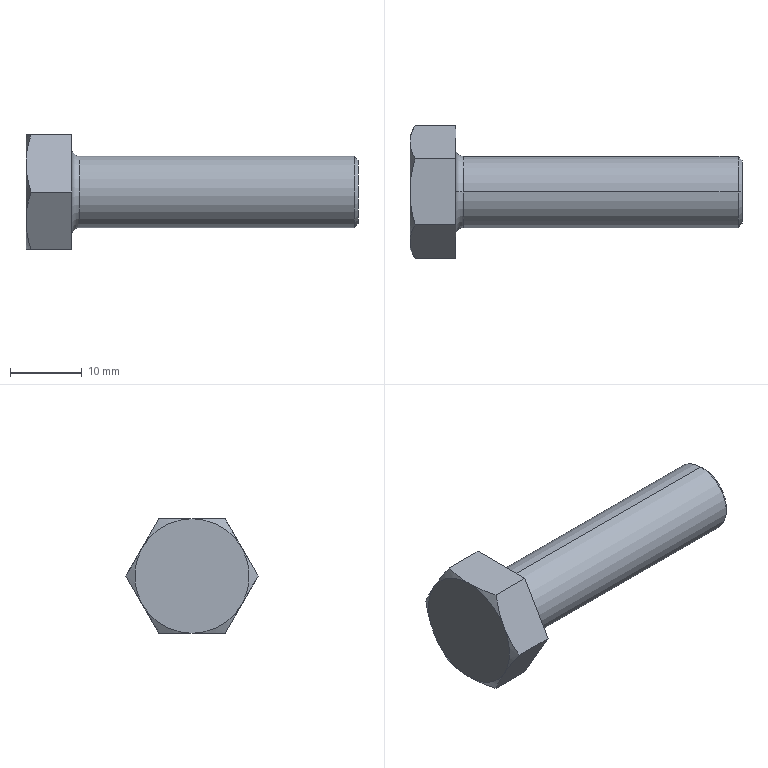Part | SolidWorks | features Chamfer 2, RevCut 2, Revolution 2, Extrusion 1, ICE 1 | 1 solid | 21 faces | box 46.4 x 18.475 x 16 mm | volume 4560 mm3 | plane 9 | cone 8 | cylinder 2 | torus 2 | commonest cylinder face diameters 10 x2
STEP:
#1=CARTESIAN_POINT('',(46.4,0.,-4.444));
#2=VERTEX_POINT('',#1);
#3=CARTESIAN_POINT('',(46.4,0.,4.444));
#4=VERTEX_POINT('',#3);
#5=CARTESIAN_POINT('',(46.4,0.,0.));
#6=DIRECTION('',(1.,0.,0.));
#7=DIRECTION('',(0.,0.,1.));
#8=AXIS2_PLACEMENT_3D('',#5,#6,#7);
#9=CIRCLE('',#8,4.444);
#10=EDGE_CURVE('',#2,#4,#9,.T.);
#11=ORIENTED_EDGE('',*,*,#10,.F.);
#12=CARTESIAN_POINT('',(45.844,0.,-5.));
#13=VERTEX_POINT('',#12);
#14=CARTESIAN_POINT('',(45.844,0.,-5.));
#15=DIRECTION('',(-0.7071,0.,-0.7071));
#16=VECTOR('',#15,1000.);
#17=LINE('',#14,#16);
#18=EDGE_CURVE('',#2,#13,#17,.T.);
#19=ORIENTED_EDGE('',*,*,#18,.T.);
#20=CARTESIAN_POINT('',(45.844,0.,5.));
#21=VERTEX_POINT('',#20);
#22=CARTESIAN_POINT('',(45.844,0.,0.));
#23=DIRECTION('',(-1.,0.,0.));
#24=DIRECTION('',(0.,0.,1.));
#25=AXIS2_PLACEMENT_3D('',#22,#23,#24);
#26=CIRCLE('',#25,5.);
#27=EDGE_CURVE('',#21,#13,#26,.T.);
#28=ORIENTED_EDGE('',*,*,#27,.F.);
#29=CARTESIAN_POINT('',(45.844,0.,5.));
#30=DIRECTION('',(-0.7071,0.,0.7071));
#31=VECTOR('',#30,1000.);
#32=LINE('',#29,#31);
#33=EDGE_CURVE('',#4,#21,#32,.T.);
#34=ORIENTED_EDGE('',*,*,#33,.F.);
#35=EDGE_LOOP('',(#11,#19,#28,#34));
#36=FACE_OUTER_BOUND('',#35,.T.);
#37=CARTESIAN_POINT('',(45.844,0.,0.));
#38=DIRECTION('',(-1.,0.,0.));
#39=DIRECTION('',(0.,0.,1.));
#40=AXIS2_PLACEMENT_3D('',#37,#38,#39);
#41=CONICAL_SURFACE('',#40,5.,0.7854);
#42=ADVANCED_FACE('',(#36),#41,.T.);
#43=ORIENTED_EDGE('',*,*,#27,.T.);
#44=CARTESIAN_POINT('',(7.5,0.,-5.));
#45=VERTEX_POINT('',#44);
#46=CARTESIAN_POINT('',(6.4,0.,-5.));
#47=DIRECTION('',(-1.,0.,0.));
#48=VECTOR('',#47,1000.);
#49=LINE('',#46,#48);
#50=EDGE_CURVE('',#13,#45,#49,.T.);
#51=ORIENTED_EDGE('',*,*,#50,.T.);
#52=CARTESIAN_POINT('',(7.5,0.,5.));
#53=VERTEX_POINT('',#52);
#54=CARTESIAN_POINT('',(7.5,0.,0.));
#55=DIRECTION('',(-1.,0.,0.));
#56=DIRECTION('',(0.,0.,1.));
#57=AXIS2_PLACEMENT_3D('',#54,#55,#56);
#58=CIRCLE('',#57,5.);
#59=EDGE_CURVE('',#53,#45,#58,.T.);
#60=ORIENTED_EDGE('',*,*,#59,.F.);
#61=CARTESIAN_POINT('',(6.4,0.,5.));
#62=DIRECTION('',(-1.,0.,0.));
#63=VECTOR('',#62,1000.);
#64=LINE('',#61,#63);
#65=EDGE_CURVE('',#21,#53,#64,.T.);
#66=ORIENTED_EDGE('',*,*,#65,.F.);
#67=EDGE_LOOP('',(#43,#51,#60,#66));
#68=FACE_OUTER_BOUND('',#67,.T.);
#69=CARTESIAN_POINT('',(6.4,0.,0.));
#70=DIRECTION('',(-1.,0.,0.));
#71=DIRECTION('',(0.,0.,1.));
#72=AXIS2_PLACEMENT_3D('',#69,#70,#71);
#73=CYLINDRICAL_SURFACE('',#72,5.);
#74=ADVANCED_FACE('',(#68),#73,.T.);
#75=CARTESIAN_POINT('',(6.4,0.,-6.1));
#76=VERTEX_POINT('',#75);
#77=CARTESIAN_POINT('',(6.4,0.,6.1));
#78=VERTEX_POINT('',#77);
#79=CARTESIAN_POINT('',(6.4,0.,0.));
#80=DIRECTION('',(-1.,0.,0.));
#81=DIRECTION('',(0.,0.,1.));
#82=AXIS2_PLACEMENT_3D('',#79,#80,#81);
#83=CIRCLE('',#82,6.1);
#84=EDGE_CURVE('',#76,#78,#83,.T.);
#85=ORIENTED_EDGE('',*,*,#84,.F.);
#86=CARTESIAN_POINT('',(7.5,0.,-6.1));
#87=DIRECTION('',(0.,1.,0.));
#88=DIRECTION('',(0.,0.,1.));
#89=AXIS2_PLACEMENT_3D('',#86,#87,#88);
#90=CIRCLE('',#89,1.1);
#91=EDGE_CURVE('',#76,#45,#90,.T.);
#92=ORIENTED_EDGE('',*,*,#91,.T.);
#93=CARTESIAN_POINT('',(7.5,0.,0.));
#94=DIRECTION('',(-1.,0.,0.));
#95=DIRECTION('',(0.,0.,1.));
#96=AXIS2_PLACEMENT_3D('',#93,#94,#95);
#97=CIRCLE('',#96,5.);
#98=EDGE_CURVE('',#45,#53,#97,.T.);
#99=ORIENTED_EDGE('',*,*,#98,.T.);
#100=CARTESIAN_POINT('',(7.5,0.,6.1));
#101=DIRECTION('',(0.,-1.,0.));
#102=DIRECTION('',(0.,0.,-1.));
#103=AXIS2_PLACEMENT_3D('',#100,#101,#102);
#104=CIRCLE('',#103,1.1);
#105=EDGE_CURVE('',#78,#53,#104,.T.);
#106=ORIENTED_EDGE('',*,*,#105,.F.);
#107=EDGE_LOOP('',(#85,#92,#99,#106));
#108=FACE_OUTER_BOUND('',#107,.T.);
#109=CARTESIAN_POINT('',(7.5,0.,0.));
#110=DIRECTION('',(-1.,0.,0.));
#111=DIRECTION('',(0.,0.,1.));
#112=AXIS2_PLACEMENT_3D('',#109,#110,#111);
#113=TOROIDAL_SURFACE('',#112,6.1,1.1);
#114=ADVANCED_FACE('',(#108),#113,.F.);
#115=CARTESIAN_POINT('',(6.4,-4.619,-8.));
#116=VERTEX_POINT('',#115);
#117=CARTESIAN_POINT('',(6.4,4.619,-8.));
#118=VERTEX_POINT('',#117);
#119=CARTESIAN_POINT('',(6.4,-4.619,-8.));
#120=DIRECTION('',(0.,1.,0.));
#121=VECTOR('',#120,1000.);
#122=LINE('',#119,#121);
#123=EDGE_CURVE('',#116,#118,#122,.T.);
#124=ORIENTED_EDGE('',*,*,#123,.T.);
#125=CARTESIAN_POINT('',(6.4,9.238,0.));
#126=VERTEX_POINT('',#125);
#127=CARTESIAN_POINT('',(6.4,4.619,-8.));
#128=DIRECTION('',(0.,0.5,0.866));
#129=VECTOR('',#128,1000.);
#130=LINE('',#127,#129);
#131=EDGE_CURVE('',#118,#126,#130,.T.);
#132=ORIENTED_EDGE('',*,*,#131,.T.);
#133=CARTESIAN_POINT('',(6.4,4.619,8.));
#134=VERTEX_POINT('',#133);
#135=CARTESIAN_POINT('',(6.4,9.238,0.));
#136=DIRECTION('',(0.,-0.5,0.866));
#137=VECTOR('',#136,1000.);
#138=LINE('',#135,#137);
#139=EDGE_CURVE('',#126,#134,#138,.T.);
#140=ORIENTED_EDGE('',*,*,#139,.T.);
#141=CARTESIAN_POINT('',(6.4,-4.619,8.));
#142=VERTEX_POINT('',#141);
#143=CARTESIAN_POINT('',(6.4,4.619,8.));
#144=DIRECTION('',(0.,-1.,0.));
#145=VECTOR('',#144,1000.);
#146=LINE('',#143,#145);
#147=EDGE_CURVE('',#134,#142,#146,.T.);
#148=ORIENTED_EDGE('',*,*,#147,.T.);
#149=CARTESIAN_POINT('',(6.4,-9.238,0.));
#150=VERTEX_POINT('',#149);
#151=CARTESIAN_POINT('',(6.4,-4.619,8.));
#152=DIRECTION('',(0.,-0.5,-0.866));
#153=VECTOR('',#152,1000.);
#154=LINE('',#151,#153);
#155=EDGE_CURVE('',#142,#150,#154,.T.);
#156=ORIENTED_EDGE('',*,*,#155,.T.);
#157=CARTESIAN_POINT('',(6.4,-9.238,0.));
#158=DIRECTION('',(0.,0.5,-0.866));
#159=VECTOR('',#158,1000.);
#160=LINE('',#157,#159);
#161=EDGE_CURVE('',#150,#116,#160,.T.);
#162=ORIENTED_EDGE('',*,*,#161,.T.);
#163=EDGE_LOOP('',(#124,#132,#140,#148,#156,#162));
#164=FACE_OUTER_BOUND('',#163,.T.);
#165=CARTESIAN_POINT('',(6.4,0.,0.));
#166=DIRECTION('',(-1.,0.,0.));
#167=DIRECTION('',(0.,0.,1.));
#168=AXIS2_PLACEMENT_3D('',#165,#166,#167);
#169=CIRCLE('',#168,6.1);
#170=EDGE_CURVE('',#78,#76,#169,.T.);
#171=ORIENTED_EDGE('',*,*,#170,.T.);
#172=ORIENTED_EDGE('',*,*,#84,.T.);
#173=EDGE_LOOP('',(#171,#172));
#174=FACE_BOUND('',#173,.T.);
#175=CARTESIAN_POINT('',(6.4,4.619,-8.));
#176=DIRECTION('',(1.,0.,0.));
#177=DIRECTION('',(0.,0.,-1.));
#178=AXIS2_PLACEMENT_3D('',#175,#176,#177);
#179=PLANE('',#178);
#180=ADVANCED_FACE('',(#164,#174),#179,.T.);
#181=CARTESIAN_POINT('',(0.7145,4.619,-8.));
#182=VERTEX_POINT('',#181);
#183=CARTESIAN_POINT('',(0.,0.,-8.));
#184=VERTEX_POINT('',#183);
#185=CARTESIAN_POINT('',(0.7145,4.619,-8.));
#186=CARTESIAN_POINT('',(0.4989,3.872,-8.));
#187=CARTESIAN_POINT('',(0.3194,3.115,-8.));
#188=CARTESIAN_POINT('',(0.06895,1.573,-8.));
#189=CARTESIAN_POINT('',(0.,0.781,-8.));
#190=CARTESIAN_POINT('',(0.,0.,-8.));
#191=B_SPLINE_CURVE_WITH_KNOTS('',3,(#185,#186,#187,#188,#189,#190),.UNSPECIFIED.,.F.,.F.,(4,2,4),(0.003372,0.005703,0.008035),.UNSPECIFIED.);
#192=EDGE_CURVE('',#182,#184,#191,.T.);
#193=ORIENTED_EDGE('',*,*,#192,.F.);
#194=CARTESIAN_POINT('',(6.4,4.619,-8.));
#195=DIRECTION('',(-1.,0.,0.));
#196=VECTOR('',#195,1000.);
#197=LINE('',#194,#196);
#198=EDGE_CURVE('',#118,#182,#197,.T.);
#199=ORIENTED_EDGE('',*,*,#198,.F.);
#200=ORIENTED_EDGE('',*,*,#123,.F.);
#201=CARTESIAN_POINT('',(0.7145,-4.619,-8.));
#202=VERTEX_POINT('',#201);
#203=CARTESIAN_POINT('',(6.4,-4.619,-8.));
#204=DIRECTION('',(-1.,0.,0.));
#205=VECTOR('',#204,1000.);
#206=LINE('',#203,#205);
#207=EDGE_CURVE('',#116,#202,#206,.T.);
#208=ORIENTED_EDGE('',*,*,#207,.T.);
#209=CARTESIAN_POINT('',(0.,0.,-8.));
#210=CARTESIAN_POINT('',(0.,-0.7805,-8.));
#211=CARTESIAN_POINT('',(0.06709,-1.556,-8.));
#212=CARTESIAN_POINT('',(0.3158,-3.098,-8.));
#213=CARTESIAN_POINT('',(0.4977,-3.868,-8.));
#214=CARTESIAN_POINT('',(0.7145,-4.619,-8.));
#215=B_SPLINE_CURVE_WITH_KNOTS('',3,(#209,#210,#211,#212,#213,#214),.UNSPECIFIED.,.F.,.F.,(4,2,4),(0.008035,0.01037,0.0127),.UNSPECIFIED.);
#216=EDGE_CURVE('',#184,#202,#215,.T.);
#217=ORIENTED_EDGE('',*,*,#216,.F.);
#218=EDGE_LOOP('',(#193,#199,#200,#208,#217));
#219=FACE_OUTER_BOUND('',#218,.T.);
#220=CARTESIAN_POINT('',(6.4,-4.619,-8.));
#221=DIRECTION('',(0.,0.,1.));
#222=DIRECTION('',(1.,0.,0.));
#223=AXIS2_PLACEMENT_3D('',#220,#221,#222);
#224=PLANE('',#223);
#225=ADVANCED_FACE('',(#219),#224,.F.);
#226=CARTESIAN_POINT('',(0.7145,9.238,0.));
#227=VERTEX_POINT('',#226);
#228=CARTESIAN_POINT('',(0.,6.928,-4.));
#229=VERTEX_POINT('',#228);
#230=CARTESIAN_POINT('',(0.7145,9.238,0.));
#231=CARTESIAN_POINT('',(0.4964,8.86,-0.6543));
#232=CARTESIAN_POINT('',(0.3167,8.479,-1.313));
#233=CARTESIAN_POINT('',(0.0681,7.71,-2.646));
#234=CARTESIAN_POINT('',(0.,7.322,-3.319));
#235=CARTESIAN_POINT('',(0.,6.928,-4.));
#236=B_SPLINE_CURVE_WITH_KNOTS('',3,(#230,#231,#232,#233,#234,#235),.UNSPECIFIED.,.F.,.F.,(4,2,4),(0.000000238,0.002337,0.004674),.UNSPECIFIED.);
#237=EDGE_CURVE('',#227,#229,#236,.T.);
#238=ORIENTED_EDGE('',*,*,#237,.F.);
#239=CARTESIAN_POINT('',(6.4,9.238,0.));
#240=DIRECTION('',(-1.,0.,0.));
#241=VECTOR('',#240,1000.);
#242=LINE('',#239,#241);
#243=EDGE_CURVE('',#126,#227,#242,.T.);
#244=ORIENTED_EDGE('',*,*,#243,.F.);
#245=ORIENTED_EDGE('',*,*,#131,.F.);
#246=ORIENTED_EDGE('',*,*,#198,.T.);
#247=CARTESIAN_POINT('',(0.,6.928,-4.));
#248=CARTESIAN_POINT('',(0.,6.732,-4.339));
#249=CARTESIAN_POINT('',(0.01689,6.535,-4.68));
#250=CARTESIAN_POINT('',(0.08225,6.146,-5.355));
#251=CARTESIAN_POINT('',(0.1307,5.952,-5.69));
#252=CARTESIAN_POINT('',(0.3174,5.376,-6.689));
#253=CARTESIAN_POINT('',(0.497,4.996,-7.347));
#254=CARTESIAN_POINT('',(0.7145,4.619,-8.));
#255=B_SPLINE_CURVE_WITH_KNOTS('',3,(#247,#248,#249,#250,#251,#252,#253,#254),.UNSPECIFIED.,.F.,.F.,(4,2,2,4),(0.004674,0.005838,0.007002,0.00933),.UNSPECIFIED.);
#256=EDGE_CURVE('',#229,#182,#255,.T.);
#257=ORIENTED_EDGE('',*,*,#256,.F.);
#258=EDGE_LOOP('',(#238,#244,#245,#246,#257));
#259=FACE_OUTER_BOUND('',#258,.T.);
#260=CARTESIAN_POINT('',(6.4,4.619,-8.));
#261=DIRECTION('',(0.,-0.866,0.5));
#262=DIRECTION('',(0.,-0.5,-0.866));
#263=AXIS2_PLACEMENT_3D('',#260,#261,#262);
#264=PLANE('',#263);
#265=ADVANCED_FACE('',(#259),#264,.F.);
#266=CARTESIAN_POINT('',(0.7145,4.619,8.));
#267=VERTEX_POINT('',#266);
#268=CARTESIAN_POINT('',(0.,6.928,4.));
#269=VERTEX_POINT('',#268);
#270=CARTESIAN_POINT('',(0.7145,4.619,8.));
#271=CARTESIAN_POINT('',(0.4964,4.997,7.346));
#272=CARTESIAN_POINT('',(0.3167,5.377,6.687));
#273=CARTESIAN_POINT('',(0.0681,6.146,5.354));
#274=CARTESIAN_POINT('',(0.,6.535,4.681));
#275=CARTESIAN_POINT('',(0.,6.928,4.));
#276=B_SPLINE_CURVE_WITH_KNOTS('',3,(#270,#271,#272,#273,#274,#275),.UNSPECIFIED.,.F.,.F.,(4,2,4),(0.000000238,0.002337,0.004674),.UNSPECIFIED.);
#277=EDGE_CURVE('',#267,#269,#276,.T.);
#278=ORIENTED_EDGE('',*,*,#277,.F.);
#279=CARTESIAN_POINT('',(6.4,4.619,8.));
#280=DIRECTION('',(-1.,0.,0.));
#281=VECTOR('',#280,1000.);
#282=LINE('',#279,#281);
#283=EDGE_CURVE('',#134,#267,#282,.T.);
#284=ORIENTED_EDGE('',*,*,#283,.F.);
#285=ORIENTED_EDGE('',*,*,#139,.F.);
#286=ORIENTED_EDGE('',*,*,#243,.T.);
#287=CARTESIAN_POINT('',(0.,6.928,4.));
#288=CARTESIAN_POINT('',(0.,7.124,3.661));
#289=CARTESIAN_POINT('',(0.01689,7.321,3.32));
#290=CARTESIAN_POINT('',(0.08225,7.711,2.645));
#291=CARTESIAN_POINT('',(0.1307,7.904,2.31));
#292=CARTESIAN_POINT('',(0.3174,8.481,1.311));
#293=CARTESIAN_POINT('',(0.497,8.861,0.6527));
#294=CARTESIAN_POINT('',(0.7145,9.238,0.));
#295=B_SPLINE_CURVE_WITH_KNOTS('',3,(#287,#288,#289,#290,#291,#292,#293,#294),.UNSPECIFIED.,.F.,.F.,(4,2,2,4),(0.004674,0.005838,0.007002,0.00933),.UNSPECIFIED.);
#296=EDGE_CURVE('',#269,#227,#295,.T.);
#297=ORIENTED_EDGE('',*,*,#296,.F.);
#298=EDGE_LOOP('',(#278,#284,#285,#286,#297));
#299=FACE_OUTER_BOUND('',#298,.T.);
#300=CARTESIAN_POINT('',(6.4,9.238,0.));
#301=DIRECTION('',(0.,-0.866,-0.5));
#302=DIRECTION('',(0.,0.5,-0.866));
#303=AXIS2_PLACEMENT_3D('',#300,#301,#302);
#304=PLANE('',#303);
#305=ADVANCED_FACE('',(#299),#304,.F.);
#306=CARTESIAN_POINT('',(0.7145,-4.619,8.));
#307=VERTEX_POINT('',#306);
#308=CARTESIAN_POINT('',(0.,0.,8.));
#309=VERTEX_POINT('',#308);
#310=CARTESIAN_POINT('',(0.7145,-4.619,8.));
#311=CARTESIAN_POINT('',(0.4977,-3.868,8.));
#312=CARTESIAN_POINT('',(0.3158,-3.098,8.));
#313=CARTESIAN_POINT('',(0.06709,-1.556,8.));
#314=CARTESIAN_POINT('',(0.,-0.7805,8.));
#315=CARTESIAN_POINT('',(0.,0.,8.));
#316=B_SPLINE_CURVE_WITH_KNOTS('',3,(#310,#311,#312,#313,#314,#315),.UNSPECIFIED.,.F.,.F.,(4,2,4),(0.008254,0.01059,0.01293),.UNSPECIFIED.);
#317=EDGE_CURVE('',#307,#309,#316,.T.);
#318=ORIENTED_EDGE('',*,*,#317,.F.);
#319=CARTESIAN_POINT('',(6.4,-4.619,8.));
#320=DIRECTION('',(-1.,0.,0.));
#321=VECTOR('',#320,1000.);
#322=LINE('',#319,#321);
#323=EDGE_CURVE('',#142,#307,#322,.T.);
#324=ORIENTED_EDGE('',*,*,#323,.F.);
#325=ORIENTED_EDGE('',*,*,#147,.F.);
#326=ORIENTED_EDGE('',*,*,#283,.T.);
#327=CARTESIAN_POINT('',(0.,0.,8.));
#328=CARTESIAN_POINT('',(0.,0.781,8.));
#329=CARTESIAN_POINT('',(0.06895,1.573,8.));
#330=CARTESIAN_POINT('',(0.3194,3.115,8.));
#331=CARTESIAN_POINT('',(0.4989,3.872,8.));
#332=CARTESIAN_POINT('',(0.7145,4.619,8.));
#333=B_SPLINE_CURVE_WITH_KNOTS('',3,(#327,#328,#329,#330,#331,#332),.UNSPECIFIED.,.F.,.F.,(4,2,4),(0.01293,0.01526,0.0176),.UNSPECIFIED.);
#334=EDGE_CURVE('',#309,#267,#333,.T.);
#335=ORIENTED_EDGE('',*,*,#334,.F.);
#336=EDGE_LOOP('',(#318,#324,#325,#326,#335));
#337=FACE_OUTER_BOUND('',#336,.T.);
#338=CARTESIAN_POINT('',(6.4,4.619,8.));
#339=DIRECTION('',(0.,0.,-1.));
#340=DIRECTION('',(0.,1.,0.));
#341=AXIS2_PLACEMENT_3D('',#338,#339,#340);
#342=PLANE('',#341);
#343=ADVANCED_FACE('',(#337),#342,.F.);
#344=CARTESIAN_POINT('',(0.7145,-9.238,0.));
#345=VERTEX_POINT('',#344);
#346=CARTESIAN_POINT('',(0.,-6.928,4.));
#347=VERTEX_POINT('',#346);
#348=CARTESIAN_POINT('',(0.7145,-9.238,0.));
#349=CARTESIAN_POINT('',(0.4964,-8.86,0.6543));
#350=CARTESIAN_POINT('',(0.3167,-8.479,1.313));
#351=CARTESIAN_POINT('',(0.0681,-7.71,2.646));
#352=CARTESIAN_POINT('',(0.,-7.322,3.319));
#353=CARTESIAN_POINT('',(0.,-6.928,4.));
#354=B_SPLINE_CURVE_WITH_KNOTS('',3,(#348,#349,#350,#351,#352,#353),.UNSPECIFIED.,.F.,.F.,(4,2,4),(0.000000238,0.002337,0.004674),.UNSPECIFIED.);
#355=EDGE_CURVE('',#345,#347,#354,.T.);
#356=ORIENTED_EDGE('',*,*,#355,.F.);
#357=CARTESIAN_POINT('',(6.4,-9.238,0.));
#358=DIRECTION('',(-1.,0.,0.));
#359=VECTOR('',#358,1000.);
#360=LINE('',#357,#359);
#361=EDGE_CURVE('',#150,#345,#360,.T.);
#362=ORIENTED_EDGE('',*,*,#361,.F.);
#363=ORIENTED_EDGE('',*,*,#155,.F.);
#364=ORIENTED_EDGE('',*,*,#323,.T.);
#365=CARTESIAN_POINT('',(0.,-6.928,4.));
#366=CARTESIAN_POINT('',(0.,-6.732,4.339));
#367=CARTESIAN_POINT('',(0.01689,-6.535,4.68));
#368=CARTESIAN_POINT('',(0.08225,-6.146,5.355));
#369=CARTESIAN_POINT('',(0.1307,-5.952,5.69));
#370=CARTESIAN_POINT('',(0.3174,-5.376,6.689));
#371=CARTESIAN_POINT('',(0.497,-4.996,7.347));
#372=CARTESIAN_POINT('',(0.7145,-4.619,8.));
#373=B_SPLINE_CURVE_WITH_KNOTS('',3,(#365,#366,#367,#368,#369,#370,#371,#372),.UNSPECIFIED.,.F.,.F.,(4,2,2,4),(0.004674,0.005838,0.007002,0.00933),.UNSPECIFIED.);
#374=EDGE_CURVE('',#347,#307,#373,.T.);
#375=ORIENTED_EDGE('',*,*,#374,.F.);
#376=EDGE_LOOP('',(#356,#362,#363,#364,#375));
#377=FACE_OUTER_BOUND('',#376,.T.);
#378=CARTESIAN_POINT('',(6.4,-4.619,8.));
#379=DIRECTION('',(0.,0.866,-0.5));
#380=DIRECTION('',(0.,0.5,0.866));
#381=AXIS2_PLACEMENT_3D('',#378,#379,#380);
#382=PLANE('',#381);
#383=ADVANCED_FACE('',(#377),#382,.F.);
#384=CARTESIAN_POINT('',(0.,-6.928,-4.));
#385=VERTEX_POINT('',#384);
#386=CARTESIAN_POINT('',(0.7145,-4.619,-8.));
#387=CARTESIAN_POINT('',(0.4964,-4.997,-7.346));
#388=CARTESIAN_POINT('',(0.3167,-5.377,-6.687));
#389=CARTESIAN_POINT('',(0.0681,-6.146,-5.354));
#390=CARTESIAN_POINT('',(0.,-6.535,-4.681));
#391=CARTESIAN_POINT('',(0.,-6.928,-4.));
#392=B_SPLINE_CURVE_WITH_KNOTS('',3,(#386,#387,#388,#389,#390,#391),.UNSPECIFIED.,.F.,.F.,(4,2,4),(0.000000238,0.002337,0.004674),.UNSPECIFIED.);
#393=EDGE_CURVE('',#202,#385,#392,.T.);
#394=ORIENTED_EDGE('',*,*,#393,.F.);
#395=ORIENTED_EDGE('',*,*,#207,.F.);
#396=ORIENTED_EDGE('',*,*,#161,.F.);
#397=ORIENTED_EDGE('',*,*,#361,.T.);
#398=CARTESIAN_POINT('',(0.,-6.928,-4.));
#399=CARTESIAN_POINT('',(0.,-7.124,-3.661));
#400=CARTESIAN_POINT('',(0.01689,-7.321,-3.32));
#401=CARTESIAN_POINT('',(0.08225,-7.711,-2.645));
#402=CARTESIAN_POINT('',(0.1307,-7.904,-2.31));
#403=CARTESIAN_POINT('',(0.3174,-8.481,-1.311));
#404=CARTESIAN_POINT('',(0.497,-8.861,-0.6527));
#405=CARTESIAN_POINT('',(0.7145,-9.238,0.));
#406=B_SPLINE_CURVE_WITH_KNOTS('',3,(#398,#399,#400,#401,#402,#403,#404,#405),.UNSPECIFIED.,.F.,.F.,(4,2,2,4),(0.004674,0.005838,0.007002,0.00933),.UNSPECIFIED.);
#407=EDGE_CURVE('',#385,#345,#406,.T.);
#408=ORIENTED_EDGE('',*,*,#407,.F.);
#409=EDGE_LOOP('',(#394,#395,#396,#397,#408));
#410=FACE_OUTER_BOUND('',#409,.T.);
#411=CARTESIAN_POINT('',(6.4,-9.238,0.));
#412=DIRECTION('',(0.,0.866,0.5));
#413=DIRECTION('',(0.,-0.5,0.866));
#414=AXIS2_PLACEMENT_3D('',#411,#412,#413);
#415=PLANE('',#414);
#416=ADVANCED_FACE('',(#410),#415,.F.);
#417=ORIENTED_EDGE('',*,*,#216,.T.);
#418=ORIENTED_EDGE('',*,*,#393,.T.);
#419=CARTESIAN_POINT('',(0.,0.,0.));
#420=DIRECTION('',(1.,0.,0.));
#421=DIRECTION('',(0.,0.,-1.));
#422=AXIS2_PLACEMENT_3D('',#419,#420,#421);
#423=CIRCLE('',#422,8.);
#424=EDGE_CURVE('',#385,#184,#423,.T.);
#425=ORIENTED_EDGE('',*,*,#424,.T.);
#426=EDGE_LOOP('',(#417,#418,#425));
#427=FACE_OUTER_BOUND('',#426,.T.);
#428=CARTESIAN_POINT('',(0.,0.,0.));
#429=DIRECTION('',(1.,0.,0.));
#430=DIRECTION('',(0.,0.,1.));
#431=AXIS2_PLACEMENT_3D('',#428,#429,#430);
#432=CONICAL_SURFACE('',#431,8.,1.047);
#433=ADVANCED_FACE('',(#427),#432,.T.);
#434=ORIENTED_EDGE('',*,*,#355,.T.);
#435=CARTESIAN_POINT('',(0.,0.,0.));
#436=DIRECTION('',(1.,0.,0.));
#437=DIRECTION('',(0.,0.,-1.));
#438=AXIS2_PLACEMENT_3D('',#435,#436,#437);
#439=CIRCLE('',#438,8.);
#440=EDGE_CURVE('',#347,#385,#439,.T.);
#441=ORIENTED_EDGE('',*,*,#440,.T.);
#442=ORIENTED_EDGE('',*,*,#407,.T.);
#443=EDGE_LOOP('',(#434,#441,#442));
#444=FACE_OUTER_BOUND('',#443,.T.);
#445=CARTESIAN_POINT('',(0.,0.,0.));
#446=DIRECTION('',(1.,0.,0.));
#447=DIRECTION('',(0.,0.,1.));
#448=AXIS2_PLACEMENT_3D('',#445,#446,#447);
#449=CONICAL_SURFACE('',#448,8.,1.047);
#450=ADVANCED_FACE('',(#444),#449,.T.);
#451=ORIENTED_EDGE('',*,*,#317,.T.);
#452=CARTESIAN_POINT('',(0.,0.,0.));
#453=DIRECTION('',(1.,0.,0.));
#454=DIRECTION('',(0.,0.,-1.));
#455=AXIS2_PLACEMENT_3D('',#452,#453,#454);
#456=CIRCLE('',#455,8.);
#457=EDGE_CURVE('',#309,#347,#456,.T.);
#458=ORIENTED_EDGE('',*,*,#457,.T.);
#459=ORIENTED_EDGE('',*,*,#374,.T.);
#460=EDGE_LOOP('',(#451,#458,#459));
#461=FACE_OUTER_BOUND('',#460,.T.);
#462=CARTESIAN_POINT('',(0.,0.,0.));
#463=DIRECTION('',(1.,0.,0.));
#464=DIRECTION('',(0.,0.,1.));
#465=AXIS2_PLACEMENT_3D('',#462,#463,#464);
#466=CONICAL_SURFACE('',#465,8.,1.047);
#467=ADVANCED_FACE('',(#461),#466,.T.);
#468=ORIENTED_EDGE('',*,*,#277,.T.);
#469=CARTESIAN_POINT('',(0.,0.,0.));
#470=DIRECTION('',(-1.,0.,0.));
#471=DIRECTION('',(0.,0.,1.));
#472=AXIS2_PLACEMENT_3D('',#469,#470,#471);
#473=CIRCLE('',#472,8.);
#474=EDGE_CURVE('',#309,#269,#473,.T.);
#475=ORIENTED_EDGE('',*,*,#474,.F.);
#476=ORIENTED_EDGE('',*,*,#334,.T.);
#477=EDGE_LOOP('',(#468,#475,#476));
#478=FACE_OUTER_BOUND('',#477,.T.);
#479=CARTESIAN_POINT('',(0.,0.,0.));
#480=DIRECTION('',(1.,0.,0.));
#481=DIRECTION('',(0.,0.,1.));
#482=AXIS2_PLACEMENT_3D('',#479,#480,#481);
#483=CONICAL_SURFACE('',#482,8.,1.047);
#484=ADVANCED_FACE('',(#478),#483,.T.);
#485=ORIENTED_EDGE('',*,*,#296,.T.);
#486=ORIENTED_EDGE('',*,*,#237,.T.);
#487=CARTESIAN_POINT('',(0.,0.,0.));
#488=DIRECTION('',(1.,0.,0.));
#489=DIRECTION('',(0.,0.,-1.));
#490=AXIS2_PLACEMENT_3D('',#487,#488,#489);
#491=CIRCLE('',#490,8.);
#492=EDGE_CURVE('',#229,#269,#491,.T.);
#493=ORIENTED_EDGE('',*,*,#492,.T.);
#494=EDGE_LOOP('',(#485,#486,#493));
#495=FACE_OUTER_BOUND('',#494,.T.);
#496=CARTESIAN_POINT('',(0.,0.,0.));
#497=DIRECTION('',(1.,0.,0.));
#498=DIRECTION('',(0.,0.,1.));
#499=AXIS2_PLACEMENT_3D('',#496,#497,#498);
#500=CONICAL_SURFACE('',#499,8.,1.047);
#501=ADVANCED_FACE('',(#495),#500,.T.);
#502=ORIENTED_EDGE('',*,*,#256,.T.);
#503=ORIENTED_EDGE('',*,*,#192,.T.);
#504=CARTESIAN_POINT('',(0.,0.,0.));
#505=DIRECTION('',(1.,0.,0.));
#506=DIRECTION('',(0.,0.,-1.));
#507=AXIS2_PLACEMENT_3D('',#504,#505,#506);
#508=CIRCLE('',#507,8.);
#509=EDGE_CURVE('',#184,#229,#508,.T.);
#510=ORIENTED_EDGE('',*,*,#509,.T.);
#511=EDGE_LOOP('',(#502,#503,#510));
#512=FACE_OUTER_BOUND('',#511,.T.);
#513=CARTESIAN_POINT('',(0.,0.,0.));
#514=DIRECTION('',(1.,0.,0.));
#515=DIRECTION('',(0.,0.,1.));
#516=AXIS2_PLACEMENT_3D('',#513,#514,#515);
#517=CONICAL_SURFACE('',#516,8.,1.047);
#518=ADVANCED_FACE('',(#512),#517,.T.);
#519=ORIENTED_EDGE('',*,*,#509,.F.);
#520=ORIENTED_EDGE('',*,*,#424,.F.);
#521=ORIENTED_EDGE('',*,*,#440,.F.);
#522=ORIENTED_EDGE('',*,*,#457,.F.);
#523=ORIENTED_EDGE('',*,*,#474,.T.);
#524=ORIENTED_EDGE('',*,*,#492,.F.);
#525=EDGE_LOOP('',(#519,#520,#521,#522,#523,#524));
#526=FACE_OUTER_BOUND('',#525,.T.);
#527=CARTESIAN_POINT('',(0.,4.619,-8.));
#528=DIRECTION('',(1.,0.,0.));
#529=DIRECTION('',(0.,0.,-1.));
#530=AXIS2_PLACEMENT_3D('',#527,#528,#529);
#531=PLANE('',#530);
#532=ADVANCED_FACE('',(#526),#531,.F.);
#533=ORIENTED_EDGE('',*,*,#91,.F.);
#534=ORIENTED_EDGE('',*,*,#170,.F.);
#535=ORIENTED_EDGE('',*,*,#105,.T.);
#536=ORIENTED_EDGE('',*,*,#59,.T.);
#537=EDGE_LOOP('',(#533,#534,#535,#536));
#538=FACE_OUTER_BOUND('',#537,.T.);
#539=CARTESIAN_POINT('',(7.5,0.,0.));
#540=DIRECTION('',(-1.,0.,0.));
#541=DIRECTION('',(0.,0.,1.));
#542=AXIS2_PLACEMENT_3D('',#539,#540,#541);
#543=TOROIDAL_SURFACE('',#542,6.1,1.1);
#544=ADVANCED_FACE('',(#538),#543,.F.);
#545=CARTESIAN_POINT('',(46.4,0.,0.));
#546=DIRECTION('',(1.,0.,0.));
#547=DIRECTION('',(0.,0.,1.));
#548=AXIS2_PLACEMENT_3D('',#545,#546,#547);
#549=CIRCLE('',#548,4.444);
#550=EDGE_CURVE('',#4,#2,#549,.T.);
#551=ORIENTED_EDGE('',*,*,#550,.T.);
#552=ORIENTED_EDGE('',*,*,#10,.T.);
#553=EDGE_LOOP('',(#551,#552));
#554=FACE_OUTER_BOUND('',#553,.T.);
#555=CARTESIAN_POINT('',(46.4,5.,0.));
#556=DIRECTION('',(-1.,0.,0.));
#557=DIRECTION('',(0.,0.,1.));
#558=AXIS2_PLACEMENT_3D('',#555,#556,#557);
#559=PLANE('',#558);
#560=ADVANCED_FACE('',(#554),#559,.F.);
#561=ORIENTED_EDGE('',*,*,#50,.F.);
#562=CARTESIAN_POINT('',(45.844,0.,0.));
#563=DIRECTION('',(-1.,0.,0.));
#564=DIRECTION('',(0.,0.,1.));
#565=AXIS2_PLACEMENT_3D('',#562,#563,#564);
#566=CIRCLE('',#565,5.);
#567=EDGE_CURVE('',#13,#21,#566,.T.);
#568=ORIENTED_EDGE('',*,*,#567,.T.);
#569=ORIENTED_EDGE('',*,*,#65,.T.);
#570=ORIENTED_EDGE('',*,*,#98,.F.);
#571=EDGE_LOOP('',(#561,#568,#569,#570));
#572=FACE_OUTER_BOUND('',#571,.T.);
#573=CARTESIAN_POINT('',(6.4,0.,0.));
#574=DIRECTION('',(-1.,0.,0.));
#575=DIRECTION('',(0.,0.,1.));
#576=AXIS2_PLACEMENT_3D('',#573,#574,#575);
#577=CYLINDRICAL_SURFACE('',#576,5.);
#578=ADVANCED_FACE('',(#572),#577,.T.);
#579=ORIENTED_EDGE('',*,*,#18,.F.);
#580=ORIENTED_EDGE('',*,*,#550,.F.);
#581=ORIENTED_EDGE('',*,*,#33,.T.);
#582=ORIENTED_EDGE('',*,*,#567,.F.);
#583=EDGE_LOOP('',(#579,#580,#581,#582));
#584=FACE_OUTER_BOUND('',#583,.T.);
#585=CARTESIAN_POINT('',(45.844,0.,0.));
#586=DIRECTION('',(-1.,0.,0.));
#587=DIRECTION('',(0.,0.,1.));
#588=AXIS2_PLACEMENT_3D('',#585,#586,#587);
#589=CONICAL_SURFACE('',#588,5.,0.7854);
#590=ADVANCED_FACE('',(#584),#589,.T.);
#591=CLOSED_SHELL('',(#42,#74,#114,#180,#225,#265,#305,#343,#383,#416,#433,#450,#467,#484,#501,#518,#532,#544,#560,#578,#590));
#592=MANIFOLD_SOLID_BREP('',#591);
#593=CARTESIAN_POINT('',(0.,0.,0.));
#594=DIRECTION('',(0.,0.,1.));
#595=DIRECTION('',(1.,0.,0.));
#596=AXIS2_PLACEMENT_3D('',#593,#594,#595);
#597=(LENGTH_UNIT()NAMED_UNIT(*)SI_UNIT(.MILLI.,.METRE.));
#598=UNCERTAINTY_MEASURE_WITH_UNIT(LENGTH_MEASURE(0.00001),#597,'','');
#599=(NAMED_UNIT(*)PLANE_ANGLE_UNIT()SI_UNIT($,.RADIAN.));
#600=(NAMED_UNIT(*)SI_UNIT($,.STERADIAN.)SOLID_ANGLE_UNIT());
#601=(GEOMETRIC_REPRESENTATION_CONTEXT(3)GLOBAL_UNCERTAINTY_ASSIGNED_CONTEXT((#598))GLOBAL_UNIT_ASSIGNED_CONTEXT((#597,#599,#600))REPRESENTATION_CONTEXT('',''));
#602=ADVANCED_BREP_SHAPE_REPRESENTATION('',(#592,#596),#601);